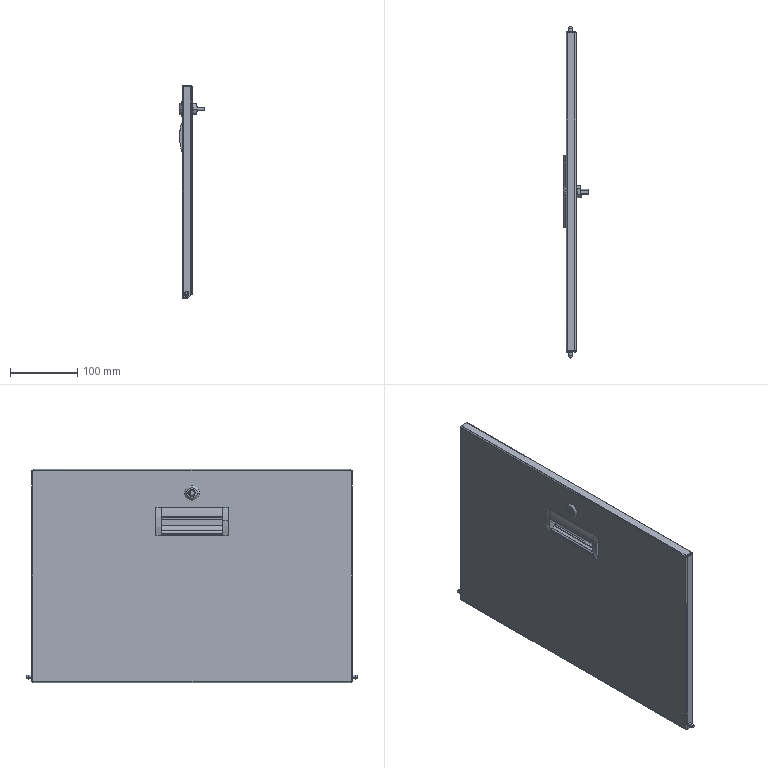Part | SolidWorks | 9 solids | 275 faces | box 37.5 x 494 x 317 mm | volume 305649 mm3 | plane 151 | cylinder 106 | spline 8 | cone 6 | torus 4 | commonest cylinder face diameters 1 x18 7 x10 5.5 x8 6 x8 0.6 x7 3.6 x7